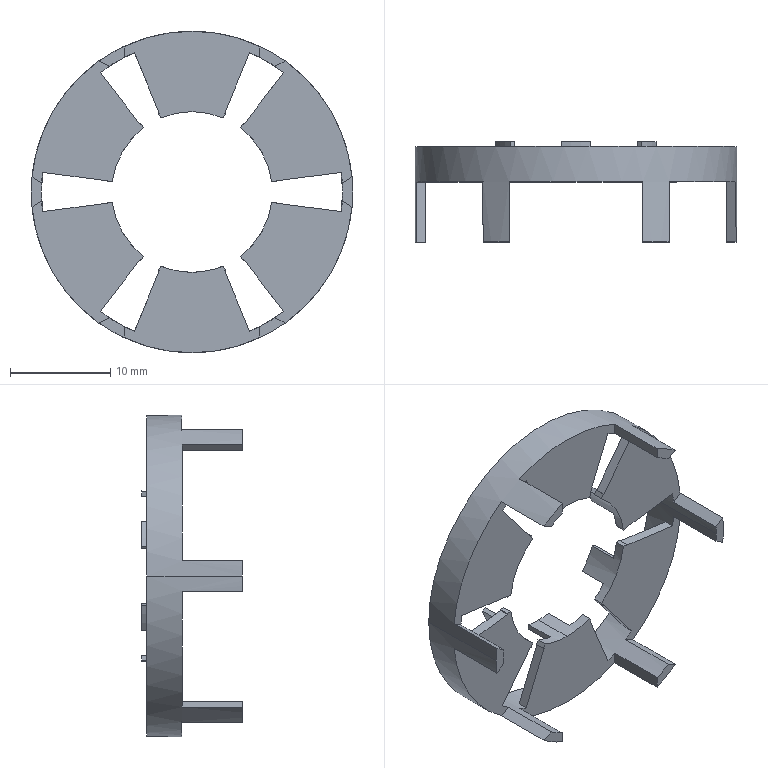Part | SolidWorks | features BaseBody 1 | 1 solid | 103 faces | box 32.009 x 10.023 x 32 mm | volume 832.245 mm3 | plane 73 | cylinder 30 | commonest cylinder face diameters 17 x19 16 x7 30 x2 32 x2